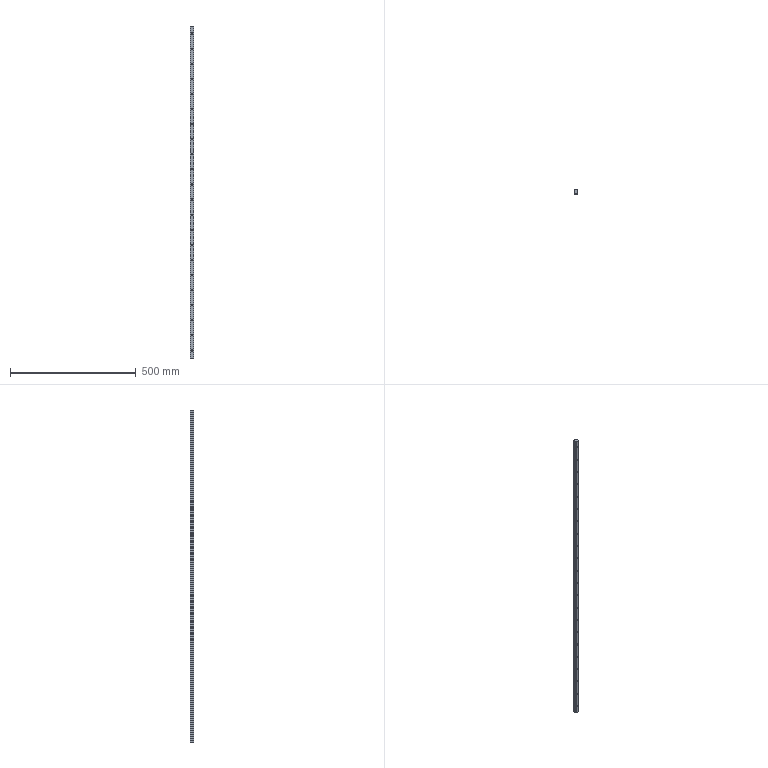Part | Creo | features CUT 23, CURVE 3, DATUM PLANE 3, COORDINATE SYSTEM 1, PATTERN 1, PROTRUSION 1 | 1 solid | 124 faces | box 14.99 x 14 x 1320 mm | volume 245585 mm3 | cylinder 90 | plane 34 | commonest cylinder face diameters 4.5 x44 7.5 x44 4.48 x2